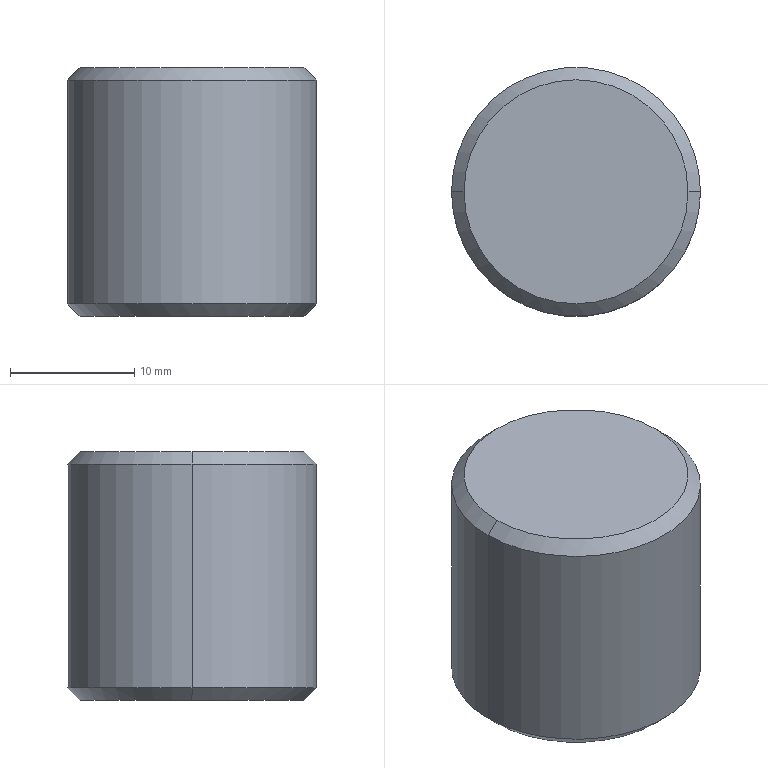Part | STEP file | SX-003-04 | 1 solid | 14 faces | box 20 x 20 x 20 mm | volume 5649 mm3 | cone 8 | cylinder 4 | plane 2 | commonest cylinder face diameters 6.8 x2 20 x2
STEP:
#1=CARTESIAN_POINT('',(0.,0.,0.));
#2=DIRECTION('',(0.,0.,1.));
#3=DIRECTION('',(1.,0.,0.));
#4=AXIS2_PLACEMENT_3D('',#1,#2,#3);
#5=CARTESIAN_POINT('',(-9.,0.,0.));
#6=VERTEX_POINT('',#5);
#7=CARTESIAN_POINT('',(9.,0.,0.));
#8=VERTEX_POINT('',#7);
#9=CARTESIAN_POINT('',(0.,0.,0.));
#10=DIRECTION('',(0.,0.,-1.));
#11=DIRECTION('',(1.,0.,0.));
#12=AXIS2_PLACEMENT_3D('',#9,#10,#11);
#13=CIRCLE('',#12,9.);
#14=CARTESIAN_POINT('',(0.,0.,1.));
#15=DIRECTION('',(0.,0.,1.));
#16=DIRECTION('',(1.,0.,0.));
#17=AXIS2_PLACEMENT_3D('',#14,#15,#16);
#18=CONICAL_SURFACE('',#17,10.,0.7854);
#19=CARTESIAN_POINT('',(6.283,-1.));
#20=DIRECTION('',(-1.,0.));
#21=VECTOR('',#20,1.);
#22=LINE('',#19,#21);
#23=(GEOMETRIC_REPRESENTATION_CONTEXT(2)PARAMETRIC_REPRESENTATION_CONTEXT()REPRESENTATION_CONTEXT('',''));
#24=DEFINITIONAL_REPRESENTATION('',(#22),#23);
#25=PCURVE('',#18,#24);
#26=CARTESIAN_POINT('',(0.,0.,0.));
#27=DIRECTION('',(0.,0.,1.));
#28=DIRECTION('',(1.,0.,0.));
#29=AXIS2_PLACEMENT_3D('',#26,#27,#28);
#30=PLANE('',#29);
#31=CARTESIAN_POINT('',(9.,0.));
#32=CARTESIAN_POINT('',(9.,-15.588));
#33=CARTESIAN_POINT('',(-4.5,-7.794));
#34=CARTESIAN_POINT('',(-18.,0.));
#35=CARTESIAN_POINT('',(-4.5,7.794));
#36=CARTESIAN_POINT('',(9.,15.588));
#37=CARTESIAN_POINT('',(9.,0.));
#38=(BOUNDED_CURVE()B_SPLINE_CURVE(2,(#31,#32,#33,#34,#35,#36,#37),.UNSPECIFIED.,.T.,.F.)B_SPLINE_CURVE_WITH_KNOTS((1,2,2,2,2,1),(-2.094,0.,2.094,4.189,6.283,8.378),.UNSPECIFIED.)CURVE()GEOMETRIC_REPRESENTATION_ITEM()RATIONAL_B_SPLINE_CURVE((1.,0.5,1.,0.5,1.,0.5,1.))REPRESENTATION_ITEM(''));
#39=(GEOMETRIC_REPRESENTATION_CONTEXT(2)PARAMETRIC_REPRESENTATION_CONTEXT()REPRESENTATION_CONTEXT('',''));
#40=DEFINITIONAL_REPRESENTATION('',(#38),#39);
#41=PCURVE('',#30,#40);
#42=SURFACE_CURVE('',#13,(#25,#41),.PCURVE_S1.);
#43=EDGE_CURVE('',#6,#8,#42,.T.);
#44=ORIENTED_EDGE('',*,*,#43,.F.);
#45=CARTESIAN_POINT('',(-10.,0.,1.));
#46=VERTEX_POINT('',#45);
#47=CARTESIAN_POINT('',(-10.,0.,1.));
#48=DIRECTION('',(-0.7071,0.,0.7071));
#49=VECTOR('',#48,1.);
#50=LINE('',#47,#49);
#51=CARTESIAN_POINT('',(3.142,0.));
#52=DIRECTION('',(0.,1.));
#53=VECTOR('',#52,1.);
#54=LINE('',#51,#53);
#55=(GEOMETRIC_REPRESENTATION_CONTEXT(2)PARAMETRIC_REPRESENTATION_CONTEXT()REPRESENTATION_CONTEXT('',''));
#56=DEFINITIONAL_REPRESENTATION('',(#54),#55);
#57=PCURVE('',#18,#56);
#58=CARTESIAN_POINT('',(0.,0.,1.));
#59=DIRECTION('',(0.,0.,1.));
#60=DIRECTION('',(1.,0.,0.));
#61=AXIS2_PLACEMENT_3D('',#58,#59,#60);
#62=CONICAL_SURFACE('',#61,10.,0.7854);
#63=CARTESIAN_POINT('',(3.142,0.));
#64=DIRECTION('',(0.,1.));
#65=VECTOR('',#64,1.);
#66=LINE('',#63,#65);
#67=(GEOMETRIC_REPRESENTATION_CONTEXT(2)PARAMETRIC_REPRESENTATION_CONTEXT()REPRESENTATION_CONTEXT('',''));
#68=DEFINITIONAL_REPRESENTATION('',(#66),#67);
#69=PCURVE('',#62,#68);
#70=SURFACE_CURVE('',#50,(#57,#69),.PCURVE_S1.);
#71=EDGE_CURVE('',#6,#46,#70,.T.);
#72=ORIENTED_EDGE('',*,*,#71,.T.);
#73=CARTESIAN_POINT('',(10.,0.,1.));
#74=VERTEX_POINT('',#73);
#75=CARTESIAN_POINT('',(0.,0.,1.));
#76=DIRECTION('',(0.,0.,1.));
#77=DIRECTION('',(1.,0.,0.));
#78=AXIS2_PLACEMENT_3D('',#75,#76,#77);
#79=CIRCLE('',#78,10.);
#80=CARTESIAN_POINT('',(0.,0.));
#81=DIRECTION('',(1.,0.));
#82=VECTOR('',#81,1.);
#83=LINE('',#80,#82);
#84=(GEOMETRIC_REPRESENTATION_CONTEXT(2)PARAMETRIC_REPRESENTATION_CONTEXT()REPRESENTATION_CONTEXT('',''));
#85=DEFINITIONAL_REPRESENTATION('',(#83),#84);
#86=PCURVE('',#18,#85);
#87=CARTESIAN_POINT('',(0.,0.,20.));
#88=DIRECTION('',(0.,0.,-1.));
#89=DIRECTION('',(-1.,0.,0.));
#90=AXIS2_PLACEMENT_3D('',#87,#88,#89);
#91=CYLINDRICAL_SURFACE('',#90,10.);
#92=CARTESIAN_POINT('',(3.142,19.));
#93=DIRECTION('',(-1.,0.));
#94=VECTOR('',#93,1.);
#95=LINE('',#92,#94);
#96=(GEOMETRIC_REPRESENTATION_CONTEXT(2)PARAMETRIC_REPRESENTATION_CONTEXT()REPRESENTATION_CONTEXT('',''));
#97=DEFINITIONAL_REPRESENTATION('',(#95),#96);
#98=PCURVE('',#91,#97);
#99=SURFACE_CURVE('',#79,(#86,#98),.PCURVE_S1.);
#100=EDGE_CURVE('',#74,#46,#99,.T.);
#101=ORIENTED_EDGE('',*,*,#100,.F.);
#102=CARTESIAN_POINT('',(10.,0.,1.));
#103=DIRECTION('',(0.7071,0.,0.7071));
#104=VECTOR('',#103,1.);
#105=LINE('',#102,#104);
#106=CARTESIAN_POINT('',(0.,0.));
#107=DIRECTION('',(0.,1.));
#108=VECTOR('',#107,1.);
#109=LINE('',#106,#108);
#110=(GEOMETRIC_REPRESENTATION_CONTEXT(2)PARAMETRIC_REPRESENTATION_CONTEXT()REPRESENTATION_CONTEXT('',''));
#111=DEFINITIONAL_REPRESENTATION('',(#109),#110);
#112=PCURVE('',#18,#111);
#113=CARTESIAN_POINT('',(6.283,0.));
#114=DIRECTION('',(0.,1.));
#115=VECTOR('',#114,1.);
#116=LINE('',#113,#115);
#117=(GEOMETRIC_REPRESENTATION_CONTEXT(2)PARAMETRIC_REPRESENTATION_CONTEXT()REPRESENTATION_CONTEXT('',''));
#118=DEFINITIONAL_REPRESENTATION('',(#116),#117);
#119=PCURVE('',#62,#118);
#120=SURFACE_CURVE('',#105,(#112,#119),.PCURVE_S1.);
#121=EDGE_CURVE('',#8,#74,#120,.T.);
#122=ORIENTED_EDGE('',*,*,#121,.F.);
#123=EDGE_LOOP('',(#44,#72,#101,#122));
#124=FACE_BOUND('',#123,.T.);
#125=ADVANCED_FACE('',(#124),#18,.T.);
#126=CARTESIAN_POINT('',(9.,0.,20.));
#127=VERTEX_POINT('',#126);
#128=CARTESIAN_POINT('',(-9.,0.,20.));
#129=VERTEX_POINT('',#128);
#130=CARTESIAN_POINT('',(0.,0.,20.));
#131=DIRECTION('',(0.,0.,1.));
#132=DIRECTION('',(1.,0.,0.));
#133=AXIS2_PLACEMENT_3D('',#130,#131,#132);
#134=CIRCLE('',#133,9.);
#135=CARTESIAN_POINT('',(0.,0.,20.));
#136=DIRECTION('',(0.,0.,-1.));
#137=DIRECTION('',(-1.,0.,0.));
#138=AXIS2_PLACEMENT_3D('',#135,#136,#137);
#139=CONICAL_SURFACE('',#138,9.,0.7854);
#140=CARTESIAN_POINT('',(3.142,0.));
#141=DIRECTION('',(-1.,0.));
#142=VECTOR('',#141,1.);
#143=LINE('',#140,#142);
#144=(GEOMETRIC_REPRESENTATION_CONTEXT(2)PARAMETRIC_REPRESENTATION_CONTEXT()REPRESENTATION_CONTEXT('',''));
#145=DEFINITIONAL_REPRESENTATION('',(#143),#144);
#146=PCURVE('',#139,#145);
#147=CARTESIAN_POINT('',(0.,0.,20.));
#148=DIRECTION('',(0.,0.,1.));
#149=DIRECTION('',(1.,0.,0.));
#150=AXIS2_PLACEMENT_3D('',#147,#148,#149);
#151=PLANE('',#150);
#152=CARTESIAN_POINT('',(0.,0.));
#153=DIRECTION('',(1.,0.));
#154=AXIS2_PLACEMENT_2D('',#152,#153);
#155=CIRCLE('',#154,9.);
#156=(GEOMETRIC_REPRESENTATION_CONTEXT(2)PARAMETRIC_REPRESENTATION_CONTEXT()REPRESENTATION_CONTEXT('',''));
#157=DEFINITIONAL_REPRESENTATION('',(#155),#156);
#158=PCURVE('',#151,#157);
#159=SURFACE_CURVE('',#134,(#146,#158),.PCURVE_S1.);
#160=EDGE_CURVE('',#127,#129,#159,.T.);
#161=ORIENTED_EDGE('',*,*,#160,.F.);
#162=CARTESIAN_POINT('',(10.,0.,19.));
#163=VERTEX_POINT('',#162);
#164=CARTESIAN_POINT('',(9.,0.,20.));
#165=DIRECTION('',(0.7071,0.,-0.7071));
#166=VECTOR('',#165,1.);
#167=LINE('',#164,#166);
#168=CARTESIAN_POINT('',(3.142,0.));
#169=DIRECTION('',(0.,1.));
#170=VECTOR('',#169,1.);
#171=LINE('',#168,#170);
#172=(GEOMETRIC_REPRESENTATION_CONTEXT(2)PARAMETRIC_REPRESENTATION_CONTEXT()REPRESENTATION_CONTEXT('',''));
#173=DEFINITIONAL_REPRESENTATION('',(#171),#172);
#174=PCURVE('',#139,#173);
#175=CARTESIAN_POINT('',(0.,0.,20.));
#176=DIRECTION('',(0.,0.,-1.));
#177=DIRECTION('',(-1.,0.,0.));
#178=AXIS2_PLACEMENT_3D('',#175,#176,#177);
#179=CONICAL_SURFACE('',#178,9.,0.7854);
#180=CARTESIAN_POINT('',(3.142,0.));
#181=DIRECTION('',(0.,1.));
#182=VECTOR('',#181,1.);
#183=LINE('',#180,#182);
#184=(GEOMETRIC_REPRESENTATION_CONTEXT(2)PARAMETRIC_REPRESENTATION_CONTEXT()REPRESENTATION_CONTEXT('',''));
#185=DEFINITIONAL_REPRESENTATION('',(#183),#184);
#186=PCURVE('',#179,#185);
#187=SURFACE_CURVE('',#167,(#174,#186),.PCURVE_S1.);
#188=EDGE_CURVE('',#127,#163,#187,.T.);
#189=ORIENTED_EDGE('',*,*,#188,.T.);
#190=CARTESIAN_POINT('',(-10.,0.,19.));
#191=VERTEX_POINT('',#190);
#192=CARTESIAN_POINT('',(0.,0.,19.));
#193=DIRECTION('',(0.,0.,-1.));
#194=DIRECTION('',(1.,0.,0.));
#195=AXIS2_PLACEMENT_3D('',#192,#193,#194);
#196=CIRCLE('',#195,10.);
#197=CARTESIAN_POINT('',(-3.142,1.));
#198=DIRECTION('',(1.,0.));
#199=VECTOR('',#198,1.);
#200=LINE('',#197,#199);
#201=(GEOMETRIC_REPRESENTATION_CONTEXT(2)PARAMETRIC_REPRESENTATION_CONTEXT()REPRESENTATION_CONTEXT('',''));
#202=DEFINITIONAL_REPRESENTATION('',(#200),#201);
#203=PCURVE('',#139,#202);
#204=CARTESIAN_POINT('',(-3.142,1.));
#205=DIRECTION('',(1.,0.));
#206=VECTOR('',#205,1.);
#207=LINE('',#204,#206);
#208=(GEOMETRIC_REPRESENTATION_CONTEXT(2)PARAMETRIC_REPRESENTATION_CONTEXT()REPRESENTATION_CONTEXT('',''));
#209=DEFINITIONAL_REPRESENTATION('',(#207),#208);
#210=PCURVE('',#91,#209);
#211=SURFACE_CURVE('',#196,(#203,#210),.PCURVE_S1.);
#212=EDGE_CURVE('',#191,#163,#211,.T.);
#213=ORIENTED_EDGE('',*,*,#212,.F.);
#214=CARTESIAN_POINT('',(-9.,0.,20.));
#215=DIRECTION('',(-0.7071,0.,-0.7071));
#216=VECTOR('',#215,1.);
#217=LINE('',#214,#216);
#218=CARTESIAN_POINT('',(0.,0.));
#219=DIRECTION('',(0.,1.));
#220=VECTOR('',#219,1.);
#221=LINE('',#218,#220);
#222=(GEOMETRIC_REPRESENTATION_CONTEXT(2)PARAMETRIC_REPRESENTATION_CONTEXT()REPRESENTATION_CONTEXT('',''));
#223=DEFINITIONAL_REPRESENTATION('',(#221),#222);
#224=PCURVE('',#139,#223);
#225=CARTESIAN_POINT('',(6.283,0.));
#226=DIRECTION('',(0.,1.));
#227=VECTOR('',#226,1.);
#228=LINE('',#225,#227);
#229=(GEOMETRIC_REPRESENTATION_CONTEXT(2)PARAMETRIC_REPRESENTATION_CONTEXT()REPRESENTATION_CONTEXT('',''));
#230=DEFINITIONAL_REPRESENTATION('',(#228),#229);
#231=PCURVE('',#179,#230);
#232=SURFACE_CURVE('',#217,(#224,#231),.PCURVE_S1.);
#233=EDGE_CURVE('',#129,#191,#232,.T.);
#234=ORIENTED_EDGE('',*,*,#233,.F.);
#235=EDGE_LOOP('',(#161,#189,#213,#234));
#236=FACE_BOUND('',#235,.T.);
#237=ADVANCED_FACE('',(#236),#139,.T.);
#238=CARTESIAN_POINT('',(-3.4,0.,0.625));
#239=VERTEX_POINT('',#238);
#240=CARTESIAN_POINT('',(-4.025,0.,0.));
#241=VERTEX_POINT('',#240);
#242=CARTESIAN_POINT('',(-4.025,0.,0.));
#243=DIRECTION('',(-0.7071,0.,-0.7071));
#244=VECTOR('',#243,1.);
#245=LINE('',#242,#244);
#246=CARTESIAN_POINT('',(0.,0.,0.));
#247=DIRECTION('',(0.,0.,-1.));
#248=DIRECTION('',(-1.,0.,0.));
#249=AXIS2_PLACEMENT_3D('',#246,#247,#248);
#250=CONICAL_SURFACE('',#249,4.025,0.7854);
#251=CARTESIAN_POINT('',(6.283,0.));
#252=DIRECTION('',(0.,1.));
#253=VECTOR('',#252,1.);
#254=LINE('',#251,#253);
#255=(GEOMETRIC_REPRESENTATION_CONTEXT(2)PARAMETRIC_REPRESENTATION_CONTEXT()REPRESENTATION_CONTEXT('',''));
#256=DEFINITIONAL_REPRESENTATION('',(#254),#255);
#257=PCURVE('',#250,#256);
#258=CARTESIAN_POINT('',(0.,0.,0.));
#259=DIRECTION('',(0.,0.,-1.));
#260=DIRECTION('',(-1.,0.,0.));
#261=AXIS2_PLACEMENT_3D('',#258,#259,#260);
#262=CONICAL_SURFACE('',#261,4.025,0.7854);
#263=CARTESIAN_POINT('',(0.,0.));
#264=DIRECTION('',(0.,1.));
#265=VECTOR('',#264,1.);
#266=LINE('',#263,#265);
#267=(GEOMETRIC_REPRESENTATION_CONTEXT(2)PARAMETRIC_REPRESENTATION_CONTEXT()REPRESENTATION_CONTEXT('',''));
#268=DEFINITIONAL_REPRESENTATION('',(#266),#267);
#269=PCURVE('',#262,#268);
#270=SURFACE_CURVE('',#245,(#257,#269),.PCURVE_S1.);
#271=EDGE_CURVE('',#239,#241,#270,.T.);
#272=ORIENTED_EDGE('',*,*,#271,.T.);
#273=CARTESIAN_POINT('',(4.025,0.,0.));
#274=VERTEX_POINT('',#273);
#275=CARTESIAN_POINT('',(0.,0.,0.));
#276=DIRECTION('',(0.,0.,-1.));
#277=DIRECTION('',(-1.,0.,0.));
#278=AXIS2_PLACEMENT_3D('',#275,#276,#277);
#279=CIRCLE('',#278,4.025);
#280=CARTESIAN_POINT('',(0.,0.));
#281=DIRECTION('',(1.,0.));
#282=VECTOR('',#281,1.);
#283=LINE('',#280,#282);
#284=(GEOMETRIC_REPRESENTATION_CONTEXT(2)PARAMETRIC_REPRESENTATION_CONTEXT()REPRESENTATION_CONTEXT('',''));
#285=DEFINITIONAL_REPRESENTATION('',(#283),#284);
#286=PCURVE('',#250,#285);
#287=CARTESIAN_POINT('',(-4.025,0.));
#288=CARTESIAN_POINT('',(-4.025,6.972));
#289=CARTESIAN_POINT('',(2.013,3.486));
#290=CARTESIAN_POINT('',(8.05,0.));
#291=CARTESIAN_POINT('',(2.013,-3.486));
#292=CARTESIAN_POINT('',(-4.025,-6.972));
#293=CARTESIAN_POINT('',(-4.025,0.));
#294=(BOUNDED_CURVE()B_SPLINE_CURVE(2,(#287,#288,#289,#290,#291,#292,#293),.UNSPECIFIED.,.T.,.F.)B_SPLINE_CURVE_WITH_KNOTS((1,2,2,2,2,1),(-2.094,0.,2.094,4.189,6.283,8.378),.UNSPECIFIED.)CURVE()GEOMETRIC_REPRESENTATION_ITEM()RATIONAL_B_SPLINE_CURVE((1.,0.5,1.,0.5,1.,0.5,1.))REPRESENTATION_ITEM(''));
#295=(GEOMETRIC_REPRESENTATION_CONTEXT(2)PARAMETRIC_REPRESENTATION_CONTEXT()REPRESENTATION_CONTEXT('',''));
#296=DEFINITIONAL_REPRESENTATION('',(#294),#295);
#297=PCURVE('',#30,#296);
#298=SURFACE_CURVE('',#279,(#286,#297),.PCURVE_S1.);
#299=EDGE_CURVE('',#274,#241,#298,.T.);
#300=ORIENTED_EDGE('',*,*,#299,.F.);
#301=CARTESIAN_POINT('',(3.4,0.,0.625));
#302=VERTEX_POINT('',#301);
#303=CARTESIAN_POINT('',(4.025,0.,0.));
#304=DIRECTION('',(0.7071,0.,-0.7071));
#305=VECTOR('',#304,1.);
#306=LINE('',#303,#305);
#307=CARTESIAN_POINT('',(3.142,0.));
#308=DIRECTION('',(0.,1.));
#309=VECTOR('',#308,1.);
#310=LINE('',#307,#309);
#311=(GEOMETRIC_REPRESENTATION_CONTEXT(2)PARAMETRIC_REPRESENTATION_CONTEXT()REPRESENTATION_CONTEXT('',''));
#312=DEFINITIONAL_REPRESENTATION('',(#310),#311);
#313=PCURVE('',#250,#312);
#314=CARTESIAN_POINT('',(3.142,0.));
#315=DIRECTION('',(0.,1.));
#316=VECTOR('',#315,1.);
#317=LINE('',#314,#316);
#318=(GEOMETRIC_REPRESENTATION_CONTEXT(2)PARAMETRIC_REPRESENTATION_CONTEXT()REPRESENTATION_CONTEXT('',''));
#319=DEFINITIONAL_REPRESENTATION('',(#317),#318);
#320=PCURVE('',#262,#319);
#321=SURFACE_CURVE('',#306,(#313,#320),.PCURVE_S1.);
#322=EDGE_CURVE('',#302,#274,#321,.T.);
#323=ORIENTED_EDGE('',*,*,#322,.F.);
#324=CARTESIAN_POINT('',(0.,0.,0.625));
#325=DIRECTION('',(0.,0.,-1.));
#326=DIRECTION('',(-1.,0.,0.));
#327=AXIS2_PLACEMENT_3D('',#324,#325,#326);
#328=CIRCLE('',#327,3.4);
#329=CARTESIAN_POINT('',(0.,-0.625));
#330=DIRECTION('',(1.,0.));
#331=VECTOR('',#330,1.);
#332=LINE('',#329,#331);
#333=(GEOMETRIC_REPRESENTATION_CONTEXT(2)PARAMETRIC_REPRESENTATION_CONTEXT()REPRESENTATION_CONTEXT('',''));
#334=DEFINITIONAL_REPRESENTATION('',(#332),#333);
#335=PCURVE('',#250,#334);
#336=CARTESIAN_POINT('',(0.,0.,0.));
#337=DIRECTION('',(0.,0.,-1.));
#338=DIRECTION('',(-1.,0.,0.));
#339=AXIS2_PLACEMENT_3D('',#336,#337,#338);
#340=CYLINDRICAL_SURFACE('',#339,3.4);
#341=CARTESIAN_POINT('',(0.,-0.625));
#342=DIRECTION('',(1.,0.));
#343=VECTOR('',#342,1.);
#344=LINE('',#341,#343);
#345=(GEOMETRIC_REPRESENTATION_CONTEXT(2)PARAMETRIC_REPRESENTATION_CONTEXT()REPRESENTATION_CONTEXT('',''));
#346=DEFINITIONAL_REPRESENTATION('',(#344),#345);
#347=PCURVE('',#340,#346);
#348=SURFACE_CURVE('',#328,(#335,#347),.PCURVE_S1.);
#349=EDGE_CURVE('',#302,#239,#348,.T.);
#350=ORIENTED_EDGE('',*,*,#349,.T.);
#351=EDGE_LOOP('',(#272,#300,#323,#350));
#352=FACE_BOUND('',#351,.F.);
#353=ADVANCED_FACE('',(#352),#250,.F.);
#354=CARTESIAN_POINT('',(-3.4,0.,15.));
#355=VERTEX_POINT('',#354);
#356=CARTESIAN_POINT('',(-3.4,0.,0.));
#357=DIRECTION('',(0.,0.,-1.));
#358=VECTOR('',#357,1.);
#359=LINE('',#356,#358);
#360=CARTESIAN_POINT('',(6.283,0.));
#361=DIRECTION('',(0.,1.));
#362=VECTOR('',#361,1.);
#363=LINE('',#360,#362);
#364=(GEOMETRIC_REPRESENTATION_CONTEXT(2)PARAMETRIC_REPRESENTATION_CONTEXT()REPRESENTATION_CONTEXT('',''));
#365=DEFINITIONAL_REPRESENTATION('',(#363),#364);
#366=PCURVE('',#340,#365);
#367=CARTESIAN_POINT('',(0.,0.,0.));
#368=DIRECTION('',(0.,0.,-1.));
#369=DIRECTION('',(-1.,0.,0.));
#370=AXIS2_PLACEMENT_3D('',#367,#368,#369);
#371=CYLINDRICAL_SURFACE('',#370,3.4);
#372=CARTESIAN_POINT('',(0.,0.));
#373=DIRECTION('',(0.,1.));
#374=VECTOR('',#373,1.);
#375=LINE('',#372,#374);
#376=(GEOMETRIC_REPRESENTATION_CONTEXT(2)PARAMETRIC_REPRESENTATION_CONTEXT()REPRESENTATION_CONTEXT('',''));
#377=DEFINITIONAL_REPRESENTATION('',(#375),#376);
#378=PCURVE('',#371,#377);
#379=SURFACE_CURVE('',#359,(#366,#378),.PCURVE_S1.);
#380=EDGE_CURVE('',#355,#239,#379,.T.);
#381=ORIENTED_EDGE('',*,*,#380,.T.);
#382=ORIENTED_EDGE('',*,*,#349,.F.);
#383=CARTESIAN_POINT('',(3.4,0.,15.));
#384=VERTEX_POINT('',#383);
#385=CARTESIAN_POINT('',(3.4,0.,0.));
#386=DIRECTION('',(0.,0.,-1.));
#387=VECTOR('',#386,1.);
#388=LINE('',#385,#387);
#389=CARTESIAN_POINT('',(3.142,0.));
#390=DIRECTION('',(0.,1.));
#391=VECTOR('',#390,1.);
#392=LINE('',#389,#391);
#393=(GEOMETRIC_REPRESENTATION_CONTEXT(2)PARAMETRIC_REPRESENTATION_CONTEXT()REPRESENTATION_CONTEXT('',''));
#394=DEFINITIONAL_REPRESENTATION('',(#392),#393);
#395=PCURVE('',#340,#394);
#396=CARTESIAN_POINT('',(3.142,0.));
#397=DIRECTION('',(0.,1.));
#398=VECTOR('',#397,1.);
#399=LINE('',#396,#398);
#400=(GEOMETRIC_REPRESENTATION_CONTEXT(2)PARAMETRIC_REPRESENTATION_CONTEXT()REPRESENTATION_CONTEXT('',''));
#401=DEFINITIONAL_REPRESENTATION('',(#399),#400);
#402=PCURVE('',#371,#401);
#403=SURFACE_CURVE('',#388,(#395,#402),.PCURVE_S1.);
#404=EDGE_CURVE('',#384,#302,#403,.T.);
#405=ORIENTED_EDGE('',*,*,#404,.F.);
#406=CARTESIAN_POINT('',(0.,0.,15.));
#407=DIRECTION('',(0.,0.,-1.));
#408=DIRECTION('',(-1.,0.,0.));
#409=AXIS2_PLACEMENT_3D('',#406,#407,#408);
#410=CIRCLE('',#409,3.4);
#411=CARTESIAN_POINT('',(0.,-15.));
#412=DIRECTION('',(1.,0.));
#413=VECTOR('',#412,1.);
#414=LINE('',#411,#413);
#415=(GEOMETRIC_REPRESENTATION_CONTEXT(2)PARAMETRIC_REPRESENTATION_CONTEXT()REPRESENTATION_CONTEXT('',''));
#416=DEFINITIONAL_REPRESENTATION('',(#414),#415);
#417=PCURVE('',#340,#416);
#418=CARTESIAN_POINT('',(0.,0.,15.));
#419=DIRECTION('',(0.,0.,-1.));
#420=DIRECTION('',(-1.,0.,0.));
#421=AXIS2_PLACEMENT_3D('',#418,#419,#420);
#422=CONICAL_SURFACE('',#421,3.4,1.03);
#423=CARTESIAN_POINT('',(0.,0.));
#424=DIRECTION('',(1.,0.));
#425=VECTOR('',#424,1.);
#426=LINE('',#423,#425);
#427=(GEOMETRIC_REPRESENTATION_CONTEXT(2)PARAMETRIC_REPRESENTATION_CONTEXT()REPRESENTATION_CONTEXT('',''));
#428=DEFINITIONAL_REPRESENTATION('',(#426),#427);
#429=PCURVE('',#422,#428);
#430=SURFACE_CURVE('',#410,(#417,#429),.PCURVE_S1.);
#431=EDGE_CURVE('',#384,#355,#430,.T.);
#432=ORIENTED_EDGE('',*,*,#431,.T.);
#433=EDGE_LOOP('',(#381,#382,#405,#432));
#434=FACE_BOUND('',#433,.F.);
#435=ADVANCED_FACE('',(#434),#340,.F.);
#436=ORIENTED_EDGE('',*,*,#431,.F.);
#437=CARTESIAN_POINT('',(0.,0.,17.043));
#438=VERTEX_POINT('',#437);
#439=CARTESIAN_POINT('',(3.4,0.,15.));
#440=DIRECTION('',(0.8572,0.,-0.515));
#441=VECTOR('',#440,1.);
#442=LINE('',#439,#441);
#443=CARTESIAN_POINT('',(3.142,0.));
#444=DIRECTION('',(0.,1.));
#445=VECTOR('',#444,1.);
#446=LINE('',#443,#445);
#447=(GEOMETRIC_REPRESENTATION_CONTEXT(2)PARAMETRIC_REPRESENTATION_CONTEXT()REPRESENTATION_CONTEXT('',''));
#448=DEFINITIONAL_REPRESENTATION('',(#446),#447);
#449=PCURVE('',#422,#448);
#450=CARTESIAN_POINT('',(0.,0.,15.));
#451=DIRECTION('',(0.,0.,-1.));
#452=DIRECTION('',(-1.,0.,0.));
#453=AXIS2_PLACEMENT_3D('',#450,#451,#452);
#454=CONICAL_SURFACE('',#453,3.4,1.03);
#455=CARTESIAN_POINT('',(3.142,0.));
#456=DIRECTION('',(0.,1.));
#457=VECTOR('',#456,1.);
#458=LINE('',#455,#457);
#459=(GEOMETRIC_REPRESENTATION_CONTEXT(2)PARAMETRIC_REPRESENTATION_CONTEXT()REPRESENTATION_CONTEXT('',''));
#460=DEFINITIONAL_REPRESENTATION('',(#458),#459);
#461=PCURVE('',#454,#460);
#462=SURFACE_CURVE('',#442,(#449,#461),.PCURVE_S1.);
#463=EDGE_CURVE('',#438,#384,#462,.T.);
#464=ORIENTED_EDGE('',*,*,#463,.F.);
#465=CARTESIAN_POINT('',(-3.4,0.,15.));
#466=DIRECTION('',(-0.8572,0.,-0.515));
#467=VECTOR('',#466,1.);
#468=LINE('',#465,#467);
#469=CARTESIAN_POINT('',(6.283,0.));
#470=DIRECTION('',(0.,1.));
#471=VECTOR('',#470,1.);
#472=LINE('',#469,#471);
#473=(GEOMETRIC_REPRESENTATION_CONTEXT(2)PARAMETRIC_REPRESENTATION_CONTEXT()REPRESENTATION_CONTEXT('',''));
#474=DEFINITIONAL_REPRESENTATION('',(#472),#473);
#475=PCURVE('',#422,#474);
#476=CARTESIAN_POINT('',(0.,0.));
#477=DIRECTION('',(0.,1.));
#478=VECTOR('',#477,1.);
#479=LINE('',#476,#478);
#480=(GEOMETRIC_REPRESENTATION_CONTEXT(2)PARAMETRIC_REPRESENTATION_CONTEXT()REPRESENTATION_CONTEXT('',''));
#481=DEFINITIONAL_REPRESENTATION('',(#479),#480);
#482=PCURVE('',#454,#481);
#483=SURFACE_CURVE('',#468,(#475,#482),.PCURVE_S1.);
#484=EDGE_CURVE('',#438,#355,#483,.T.);
#485=ORIENTED_EDGE('',*,*,#484,.T.);
#486=EDGE_LOOP('',(#436,#464,#485));
#487=FACE_BOUND('',#486,.F.);
#488=ADVANCED_FACE('',(#487),#422,.F.);
#489=ORIENTED_EDGE('',*,*,#212,.T.);
#490=CARTESIAN_POINT('',(10.,0.,20.));
#491=DIRECTION('',(0.,0.,-1.));
#492=VECTOR('',#491,1.);
#493=LINE('',#490,#492);
#494=CARTESIAN_POINT('',(3.142,0.));
#495=DIRECTION('',(0.,1.));
#496=VECTOR('',#495,1.);
#497=LINE('',#494,#496);
#498=(GEOMETRIC_REPRESENTATION_CONTEXT(2)PARAMETRIC_REPRESENTATION_CONTEXT()REPRESENTATION_CONTEXT('',''));
#499=DEFINITIONAL_REPRESENTATION('',(#497),#498);
#500=PCURVE('',#91,#499);
#501=CARTESIAN_POINT('',(0.,0.,20.));
#502=DIRECTION('',(0.,0.,-1.));
#503=DIRECTION('',(-1.,0.,0.));
#504=AXIS2_PLACEMENT_3D('',#501,#502,#503);
#505=CYLINDRICAL_SURFACE('',#504,10.);
#506=CARTESIAN_POINT('',(3.142,0.));
#507=DIRECTION('',(0.,1.));
#508=VECTOR('',#507,1.);
#509=LINE('',#506,#508);
#510=(GEOMETRIC_REPRESENTATION_CONTEXT(2)PARAMETRIC_REPRESENTATION_CONTEXT()REPRESENTATION_CONTEXT('',''));
#511=DEFINITIONAL_REPRESENTATION('',(#509),#510);
#512=PCURVE('',#505,#511);
#513=SURFACE_CURVE('',#493,(#500,#512),.PCURVE_S1.);
#514=EDGE_CURVE('',#163,#74,#513,.T.);
#515=ORIENTED_EDGE('',*,*,#514,.T.);
#516=ORIENTED_EDGE('',*,*,#100,.T.);
#517=CARTESIAN_POINT('',(-10.,0.,20.));
#518=DIRECTION('',(0.,0.,-1.));
#519=VECTOR('',#518,1.);
#520=LINE('',#517,#519);
#521=CARTESIAN_POINT('',(0.,0.));
#522=DIRECTION('',(0.,1.));
#523=VECTOR('',#522,1.);
#524=LINE('',#521,#523);
#525=(GEOMETRIC_REPRESENTATION_CONTEXT(2)PARAMETRIC_REPRESENTATION_CONTEXT()REPRESENTATION_CONTEXT('',''));
#526=DEFINITIONAL_REPRESENTATION('',(#524),#525);
#527=PCURVE('',#91,#526);
#528=CARTESIAN_POINT('',(6.283,0.));
#529=DIRECTION('',(0.,1.));
#530=VECTOR('',#529,1.);
#531=LINE('',#528,#530);
#532=(GEOMETRIC_REPRESENTATION_CONTEXT(2)PARAMETRIC_REPRESENTATION_CONTEXT()REPRESENTATION_CONTEXT('',''));
#533=DEFINITIONAL_REPRESENTATION('',(#531),#532);
#534=PCURVE('',#505,#533);
#535=SURFACE_CURVE('',#520,(#527,#534),.PCURVE_S1.);
#536=EDGE_CURVE('',#191,#46,#535,.T.);
#537=ORIENTED_EDGE('',*,*,#536,.F.);
#538=EDGE_LOOP('',(#489,#515,#516,#537));
#539=FACE_BOUND('',#538,.T.);
#540=ADVANCED_FACE('',(#539),#91,.T.);
#541=ORIENTED_EDGE('',*,*,#514,.F.);
#542=CARTESIAN_POINT('',(0.,0.,19.));
#543=DIRECTION('',(0.,0.,-1.));
#544=DIRECTION('',(1.,0.,0.));
#545=AXIS2_PLACEMENT_3D('',#542,#543,#544);
#546=CIRCLE('',#545,10.);
#547=CARTESIAN_POINT('',(3.142,1.));
#548=DIRECTION('',(1.,0.));
#549=VECTOR('',#548,1.);
#550=LINE('',#547,#549);
#551=(GEOMETRIC_REPRESENTATION_CONTEXT(2)PARAMETRIC_REPRESENTATION_CONTEXT()REPRESENTATION_CONTEXT('',''));
#552=DEFINITIONAL_REPRESENTATION('',(#550),#551);
#553=PCURVE('',#505,#552);
#554=CARTESIAN_POINT('',(3.142,1.));
#555=DIRECTION('',(1.,0.));
#556=VECTOR('',#555,1.);
#557=LINE('',#554,#556);
#558=(GEOMETRIC_REPRESENTATION_CONTEXT(2)PARAMETRIC_REPRESENTATION_CONTEXT()REPRESENTATION_CONTEXT('',''));
#559=DEFINITIONAL_REPRESENTATION('',(#557),#558);
#560=PCURVE('',#179,#559);
#561=SURFACE_CURVE('',#546,(#553,#560),.PCURVE_S1.);
#562=EDGE_CURVE('',#163,#191,#561,.T.);
#563=ORIENTED_EDGE('',*,*,#562,.T.);
#564=ORIENTED_EDGE('',*,*,#536,.T.);
#565=CARTESIAN_POINT('',(0.,0.,1.));
#566=DIRECTION('',(0.,0.,1.));
#567=DIRECTION('',(1.,0.,0.));
#568=AXIS2_PLACEMENT_3D('',#565,#566,#567);
#569=CIRCLE('',#568,10.);
#570=CARTESIAN_POINT('',(9.425,19.));
#571=DIRECTION('',(-1.,0.));
#572=VECTOR('',#571,1.);
#573=LINE('',#570,#572);
#574=(GEOMETRIC_REPRESENTATION_CONTEXT(2)PARAMETRIC_REPRESENTATION_CONTEXT()REPRESENTATION_CONTEXT('',''));
#575=DEFINITIONAL_REPRESENTATION('',(#573),#574);
#576=PCURVE('',#505,#575);
#577=CARTESIAN_POINT('',(0.,0.));
#578=DIRECTION('',(1.,0.));
#579=VECTOR('',#578,1.);
#580=LINE('',#577,#579);
#581=(GEOMETRIC_REPRESENTATION_CONTEXT(2)PARAMETRIC_REPRESENTATION_CONTEXT()REPRESENTATION_CONTEXT('',''));
#582=DEFINITIONAL_REPRESENTATION('',(#580),#581);
#583=PCURVE('',#62,#582);
#584=SURFACE_CURVE('',#569,(#576,#583),.PCURVE_S1.);
#585=EDGE_CURVE('',#46,#74,#584,.T.);
#586=ORIENTED_EDGE('',*,*,#585,.T.);
#587=EDGE_LOOP('',(#541,#563,#564,#586));
#588=FACE_BOUND('',#587,.T.);
#589=ADVANCED_FACE('',(#588),#505,.T.);
#590=CARTESIAN_POINT('',(0.,0.,20.));
#591=DIRECTION('',(0.,0.,1.));
#592=DIRECTION('',(1.,0.,0.));
#593=AXIS2_PLACEMENT_3D('',#590,#591,#592);
#594=CIRCLE('',#593,9.);
#595=CARTESIAN_POINT('',(0.,0.));
#596=DIRECTION('',(1.,0.));
#597=AXIS2_PLACEMENT_2D('',#595,#596);
#598=CIRCLE('',#597,9.);
#599=(GEOMETRIC_REPRESENTATION_CONTEXT(2)PARAMETRIC_REPRESENTATION_CONTEXT()REPRESENTATION_CONTEXT('',''));
#600=DEFINITIONAL_REPRESENTATION('',(#598),#599);
#601=PCURVE('',#151,#600);
#602=CARTESIAN_POINT('',(9.425,0.));
#603=DIRECTION('',(-1.,0.));
#604=VECTOR('',#603,1.);
#605=LINE('',#602,#604);
#606=(GEOMETRIC_REPRESENTATION_CONTEXT(2)PARAMETRIC_REPRESENTATION_CONTEXT()REPRESENTATION_CONTEXT('',''));
#607=DEFINITIONAL_REPRESENTATION('',(#605),#606);
#608=PCURVE('',#179,#607);
#609=SURFACE_CURVE('',#594,(#601,#608),.PCURVE_S1.);
#610=EDGE_CURVE('',#129,#127,#609,.T.);
#611=ORIENTED_EDGE('',*,*,#610,.T.);
#612=ORIENTED_EDGE('',*,*,#160,.T.);
#613=EDGE_LOOP('',(#611,#612));
#614=FACE_BOUND('',#613,.T.);
#615=ADVANCED_FACE('',(#614),#151,.T.);
#616=CARTESIAN_POINT('',(0.,0.,0.));
#617=DIRECTION('',(0.,0.,-1.));
#618=DIRECTION('',(1.,0.,0.));
#619=AXIS2_PLACEMENT_3D('',#616,#617,#618);
#620=CIRCLE('',#619,9.);
#621=CARTESIAN_POINT('',(9.,0.));
#622=CARTESIAN_POINT('',(9.,-15.588));
#623=CARTESIAN_POINT('',(-4.5,-7.794));
#624=CARTESIAN_POINT('',(-18.,0.));
#625=CARTESIAN_POINT('',(-4.5,7.794));
#626=CARTESIAN_POINT('',(9.,15.588));
#627=CARTESIAN_POINT('',(9.,0.));
#628=(BOUNDED_CURVE()B_SPLINE_CURVE(2,(#621,#622,#623,#624,#625,#626,#627),.UNSPECIFIED.,.T.,.F.)B_SPLINE_CURVE_WITH_KNOTS((1,2,2,2,2,1),(-2.094,0.,2.094,4.189,6.283,8.378),.UNSPECIFIED.)CURVE()GEOMETRIC_REPRESENTATION_ITEM()RATIONAL_B_SPLINE_CURVE((1.,0.5,1.,0.5,1.,0.5,1.))REPRESENTATION_ITEM(''));
#629=(GEOMETRIC_REPRESENTATION_CONTEXT(2)PARAMETRIC_REPRESENTATION_CONTEXT()REPRESENTATION_CONTEXT('',''));
#630=DEFINITIONAL_REPRESENTATION('',(#628),#629);
#631=PCURVE('',#30,#630);
#632=CARTESIAN_POINT('',(6.283,-1.));
#633=DIRECTION('',(-1.,0.));
#634=VECTOR('',#633,1.);
#635=LINE('',#632,#634);
#636=(GEOMETRIC_REPRESENTATION_CONTEXT(2)PARAMETRIC_REPRESENTATION_CONTEXT()REPRESENTATION_CONTEXT('',''));
#637=DEFINITIONAL_REPRESENTATION('',(#635),#636);
#638=PCURVE('',#62,#637);
#639=SURFACE_CURVE('',#620,(#631,#638),.PCURVE_S1.);
#640=EDGE_CURVE('',#8,#6,#639,.T.);
#641=ORIENTED_EDGE('',*,*,#640,.T.);
#642=ORIENTED_EDGE('',*,*,#43,.T.);
#643=EDGE_LOOP('',(#641,#642));
#644=FACE_BOUND('',#643,.T.);
#645=CARTESIAN_POINT('',(0.,0.,0.));
#646=DIRECTION('',(0.,0.,-1.));
#647=DIRECTION('',(-1.,0.,0.));
#648=AXIS2_PLACEMENT_3D('',#645,#646,#647);
#649=CIRCLE('',#648,4.025);
#650=CARTESIAN_POINT('',(-4.025,0.));
#651=CARTESIAN_POINT('',(-4.025,6.972));
#652=CARTESIAN_POINT('',(2.013,3.486));
#653=CARTESIAN_POINT('',(8.05,0.));
#654=CARTESIAN_POINT('',(2.013,-3.486));
#655=CARTESIAN_POINT('',(-4.025,-6.972));
#656=CARTESIAN_POINT('',(-4.025,0.));
#657=(BOUNDED_CURVE()B_SPLINE_CURVE(2,(#650,#651,#652,#653,#654,#655,#656),.UNSPECIFIED.,.T.,.F.)B_SPLINE_CURVE_WITH_KNOTS((1,2,2,2,2,1),(-2.094,0.,2.094,4.189,6.283,8.378),.UNSPECIFIED.)CURVE()GEOMETRIC_REPRESENTATION_ITEM()RATIONAL_B_SPLINE_CURVE((1.,0.5,1.,0.5,1.,0.5,1.))REPRESENTATION_ITEM(''));
#658=(GEOMETRIC_REPRESENTATION_CONTEXT(2)PARAMETRIC_REPRESENTATION_CONTEXT()REPRESENTATION_CONTEXT('',''));
#659=DEFINITIONAL_REPRESENTATION('',(#657),#658);
#660=PCURVE('',#30,#659);
#661=CARTESIAN_POINT('',(0.,0.));
#662=DIRECTION('',(1.,0.));
#663=VECTOR('',#662,1.);
#664=LINE('',#661,#663);
#665=(GEOMETRIC_REPRESENTATION_CONTEXT(2)PARAMETRIC_REPRESENTATION_CONTEXT()REPRESENTATION_CONTEXT('',''));
#666=DEFINITIONAL_REPRESENTATION('',(#664),#665);
#667=PCURVE('',#262,#666);
#668=SURFACE_CURVE('',#649,(#660,#667),.PCURVE_S1.);
#669=EDGE_CURVE('',#241,#274,#668,.T.);
#670=ORIENTED_EDGE('',*,*,#669,.F.);
#671=ORIENTED_EDGE('',*,*,#299,.F.);
#672=EDGE_LOOP('',(#670,#671));
#673=FACE_BOUND('',#672,.T.);
#674=ADVANCED_FACE('',(#644,#673),#30,.F.);
#675=CARTESIAN_POINT('',(0.,0.,15.));
#676=DIRECTION('',(0.,0.,-1.));
#677=DIRECTION('',(-1.,0.,0.));
#678=AXIS2_PLACEMENT_3D('',#675,#676,#677);
#679=CIRCLE('',#678,3.4);
#680=CARTESIAN_POINT('',(0.,0.));
#681=DIRECTION('',(1.,0.));
#682=VECTOR('',#681,1.);
#683=LINE('',#680,#682);
#684=(GEOMETRIC_REPRESENTATION_CONTEXT(2)PARAMETRIC_REPRESENTATION_CONTEXT()REPRESENTATION_CONTEXT('',''));
#685=DEFINITIONAL_REPRESENTATION('',(#683),#684);
#686=PCURVE('',#454,#685);
#687=CARTESIAN_POINT('',(0.,-15.));
#688=DIRECTION('',(1.,0.));
#689=VECTOR('',#688,1.);
#690=LINE('',#687,#689);
#691=(GEOMETRIC_REPRESENTATION_CONTEXT(2)PARAMETRIC_REPRESENTATION_CONTEXT()REPRESENTATION_CONTEXT('',''));
#692=DEFINITIONAL_REPRESENTATION('',(#690),#691);
#693=PCURVE('',#371,#692);
#694=SURFACE_CURVE('',#679,(#686,#693),.PCURVE_S1.);
#695=EDGE_CURVE('',#355,#384,#694,.T.);
#696=ORIENTED_EDGE('',*,*,#695,.F.);
#697=ORIENTED_EDGE('',*,*,#484,.F.);
#698=ORIENTED_EDGE('',*,*,#463,.T.);
#699=EDGE_LOOP('',(#696,#697,#698));
#700=FACE_BOUND('',#699,.F.);
#701=ADVANCED_FACE('',(#700),#454,.F.);
#702=CARTESIAN_POINT('',(0.,0.,0.625));
#703=DIRECTION('',(0.,0.,-1.));
#704=DIRECTION('',(-1.,0.,0.));
#705=AXIS2_PLACEMENT_3D('',#702,#703,#704);
#706=CIRCLE('',#705,3.4);
#707=CARTESIAN_POINT('',(0.,-0.625));
#708=DIRECTION('',(1.,0.));
#709=VECTOR('',#708,1.);
#710=LINE('',#707,#709);
#711=(GEOMETRIC_REPRESENTATION_CONTEXT(2)PARAMETRIC_REPRESENTATION_CONTEXT()REPRESENTATION_CONTEXT('',''));
#712=DEFINITIONAL_REPRESENTATION('',(#710),#711);
#713=PCURVE('',#371,#712);
#714=CARTESIAN_POINT('',(0.,-0.625));
#715=DIRECTION('',(1.,0.));
#716=VECTOR('',#715,1.);
#717=LINE('',#714,#716);
#718=(GEOMETRIC_REPRESENTATION_CONTEXT(2)PARAMETRIC_REPRESENTATION_CONTEXT()REPRESENTATION_CONTEXT('',''));
#719=DEFINITIONAL_REPRESENTATION('',(#717),#718);
#720=PCURVE('',#262,#719);
#721=SURFACE_CURVE('',#706,(#713,#720),.PCURVE_S1.);
#722=EDGE_CURVE('',#239,#302,#721,.T.);
#723=ORIENTED_EDGE('',*,*,#722,.F.);
#724=ORIENTED_EDGE('',*,*,#380,.F.);
#725=ORIENTED_EDGE('',*,*,#695,.T.);
#726=ORIENTED_EDGE('',*,*,#404,.T.);
#727=EDGE_LOOP('',(#723,#724,#725,#726));
#728=FACE_BOUND('',#727,.F.);
#729=ADVANCED_FACE('',(#728),#371,.F.);
#730=ORIENTED_EDGE('',*,*,#669,.F.);
#731=ORIENTED_EDGE('',*,*,#271,.F.);
#732=ORIENTED_EDGE('',*,*,#722,.T.);
#733=ORIENTED_EDGE('',*,*,#322,.T.);
#734=EDGE_LOOP('',(#730,#731,#732,#733));
#735=FACE_BOUND('',#734,.F.);
#736=ADVANCED_FACE('',(#735),#262,.F.);
#737=ORIENTED_EDGE('',*,*,#188,.F.);
#738=ORIENTED_EDGE('',*,*,#610,.F.);
#739=ORIENTED_EDGE('',*,*,#233,.T.);
#740=ORIENTED_EDGE('',*,*,#562,.F.);
#741=EDGE_LOOP('',(#737,#738,#739,#740));
#742=FACE_BOUND('',#741,.T.);
#743=ADVANCED_FACE('',(#742),#179,.T.);
#744=ORIENTED_EDGE('',*,*,#71,.F.);
#745=ORIENTED_EDGE('',*,*,#640,.F.);
#746=ORIENTED_EDGE('',*,*,#121,.T.);
#747=ORIENTED_EDGE('',*,*,#585,.F.);
#748=EDGE_LOOP('',(#744,#745,#746,#747));
#749=FACE_BOUND('',#748,.T.);
#750=ADVANCED_FACE('',(#749),#62,.T.);
#751=CLOSED_SHELL('',(#125,#237,#353,#435,#488,#540,#589,#615,#674,#701,#729,#736,#743,#750));
#752=MANIFOLD_SOLID_BREP('',#751);
#753=(LENGTH_UNIT()NAMED_UNIT(*)SI_UNIT(.MILLI.,.METRE.));
#754=UNCERTAINTY_MEASURE_WITH_UNIT(LENGTH_MEASURE(0.0000001),#753,'','');
#755=(NAMED_UNIT(*)PLANE_ANGLE_UNIT()SI_UNIT($,.RADIAN.));
#756=(NAMED_UNIT(*)SI_UNIT($,.STERADIAN.)SOLID_ANGLE_UNIT());
#757=(GEOMETRIC_REPRESENTATION_CONTEXT(3)GLOBAL_UNCERTAINTY_ASSIGNED_CONTEXT((#754))GLOBAL_UNIT_ASSIGNED_CONTEXT((#753,#755,#756))REPRESENTATION_CONTEXT('',''));
#758=ADVANCED_BREP_SHAPE_REPRESENTATION('',(#4,#752),#757);